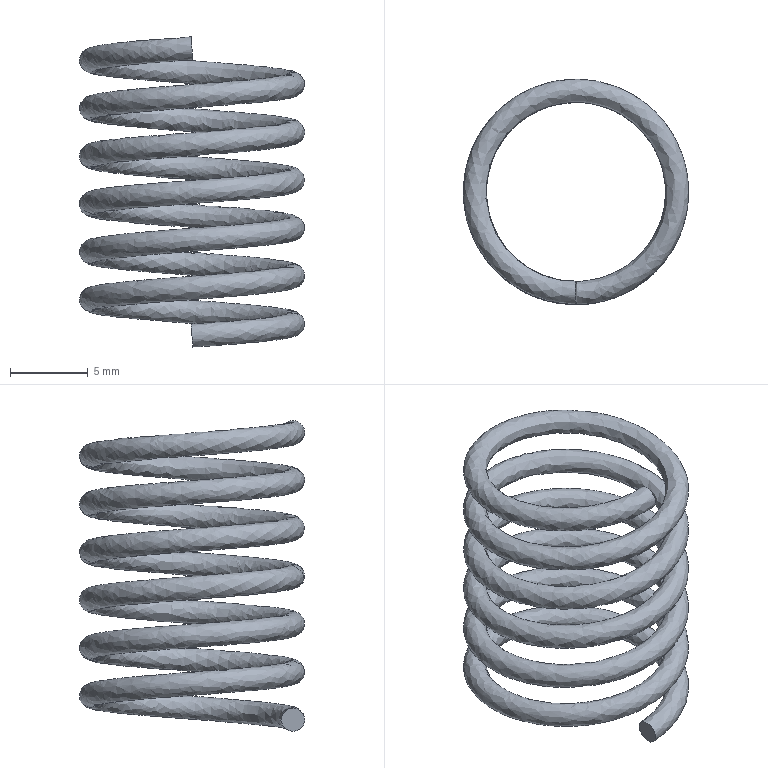Part | STEP file | 1-01.10 | 1 solid | 3 faces | box 14.501 x 14.501 x 19.996 mm | volume 434.428 mm3 | plane 2 | spline 1